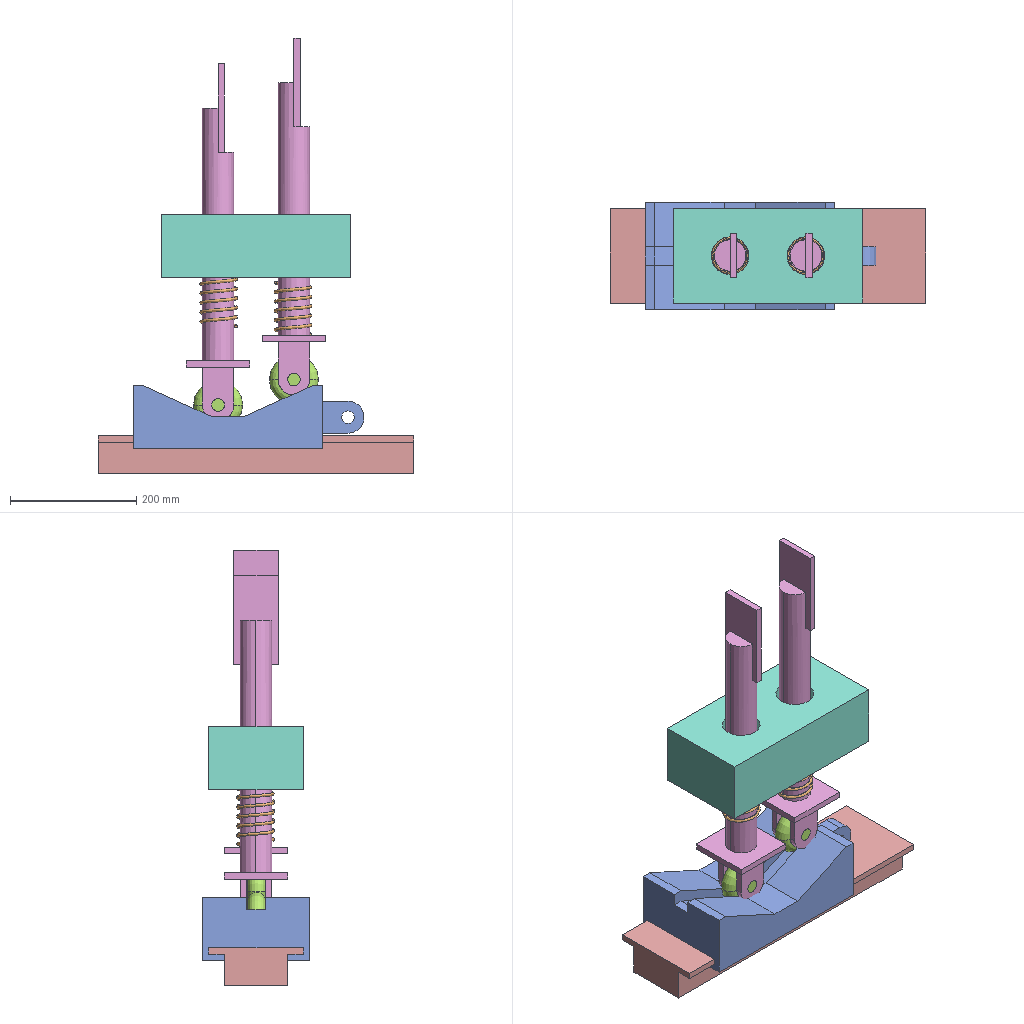Assembly | SolidWorks | 6 different items | 9 placed | box 500 x 170 x 689 mm
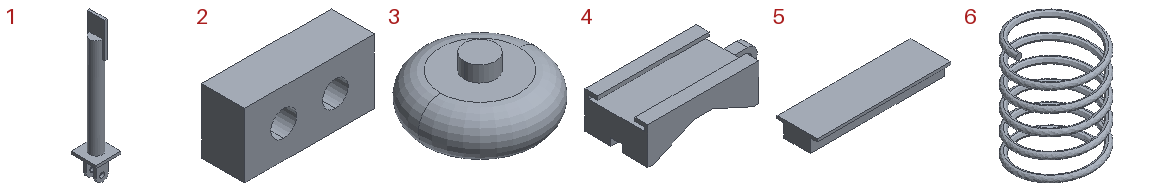Parts list (item | quantity | size | volume | features):
1 | x2 | 100 x 100 x 565 mm | 988028 mm3 | features ICE 5, Extrusion 1
2 | x1 | 300 x 100 x 150 mm | 3934513 mm3 | features Extrusion 1
3 | x2 | 78.234 x 78.234 x 50 mm | 123364 mm3 | features Extrusion 1, Revolution 1
4 | x1 | 365.5 x 170 x 100 mm | 2892418 mm3 | features ICE 5, MirrorPattern 2, Extrusion 1
5 | x1 | 500 x 150 x 60 mm | 3250000 mm3 | features Extrusion 1, ICE 1
6 | x2 | 60 x 60 x 86.725 mm | 15240 mm3 | features Helix 1, Sweep 1
Mates (type | each side: item.copy, entity, surface, feature):
Coincident | 5.1 face plane Boss-Extrude1 | 4.1 face plane Boss-Extrude1
Width | 4.1 face plane Boss-Extrude1 | 4.1 face plane Boss-Extrude1 | 5.1 face plane Boss-Extrude2 | 5.1 face plane Boss-Extrude2
Concentric | assembly face | assembly face
Coincident | assembly face | assembly face
Width | assembly face | assembly face | 4.1 face plane Cut-Extrude1 | 4.1 face plane Cut-Extrude1
Tangent | 4.1 face plane Cut-Extrude1 | assembly face
Concentric | 3.1 face cylinder Boss-Extrude1 | 1.1 face cylinder Boss-Extrude2
Coincident | 3.1 face plane Boss-Extrude1 | 1.1 face plane Boss-Extrude2
Width | 4.1 face plane Boss-Extrude1 | 4.1 face plane Boss-Extrude1 | 1.1 face plane Boss-Extrude2 | 1.1 face plane Boss-Extrude2
Tangent | 4.1 face plane Cut-Extrude1 | 3.1 face torus Revolve3
Concentric | 1.1 face cylinder Boss-Extrude3 | 2.1 face cylinder Boss-Extrude1
Coincident | 1.2 face plane Boss-Extrude2 | 3.2 edge
Concentric | 1.2 face cylinder Boss-Extrude2 | 3.2 face cylinder Boss-Extrude1
Width | 1.2 face plane Boss-Extrude2 | 1.2 face plane Boss-Extrude2 | 4.1 face plane Boss-Extrude1 | 4.1 face plane Boss-Extrude1
Tangent | 4.1 face plane Mirror2 | 3.2 face torus Revolve3
Concentric | 2.1 face cylinder Boss-Extrude1 | 1.2 face cylinder Boss-Extrude3
Width | 2.1 face plane Boss-Extrude1 | 2.1 face plane Boss-Extrude1 | 5.1 face plane Boss-Extrude2 | 5.1 face plane Boss-Extrude2
Width | 2.1 face plane Boss-Extrude1 | 2.1 face plane Boss-Extrude1 | 5.1 face plane Boss-Extrude1 | 5.1 face plane Boss-Extrude1
DistanceDim | 5.1 face plane Boss-Extrude1 | 2.1 face plane Boss-Extrude1